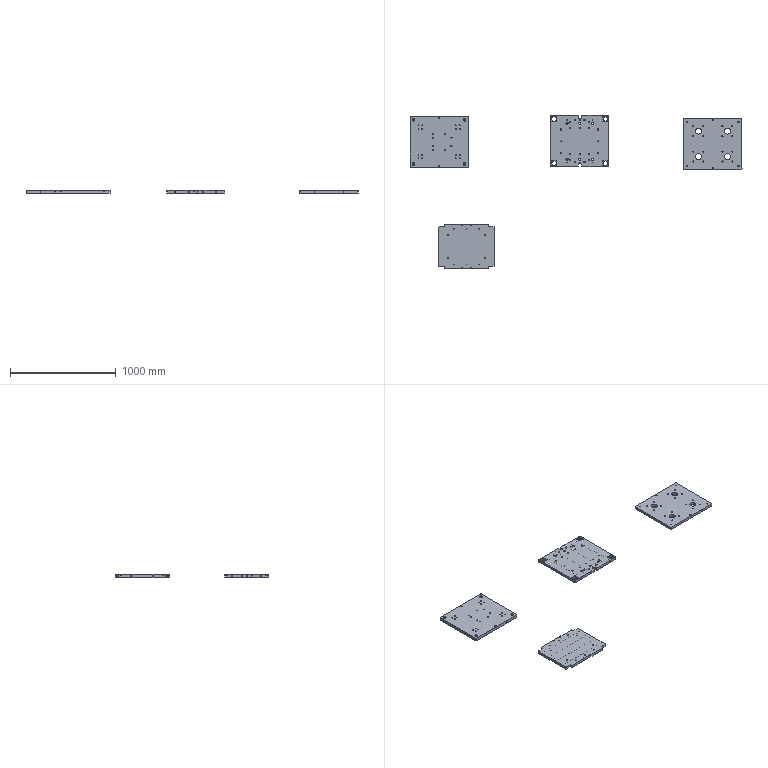Part | 4 solids | 518 faces | box 3140 x 1452 x 30 mm | volume 25671833 mm3 | cylinder 414 | plane 104 | commonest cylinder face diameters 5.2 x100 10.5 x72 10 x44 9 x40 5.5 x32 11 x20